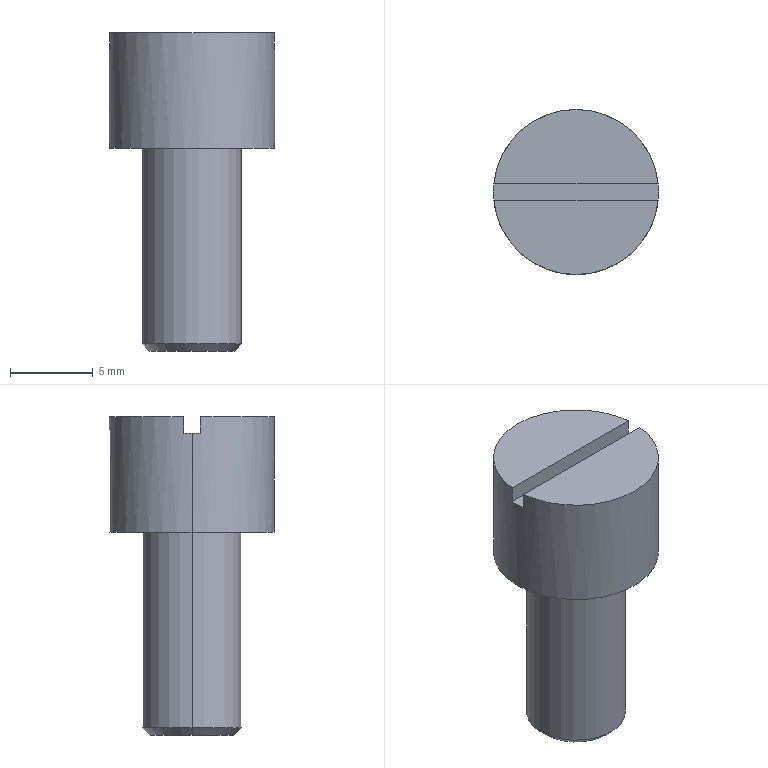Part | Creo | 1 solid | 13 faces | box 10 x 10 x 19.3 mm | volume 885.757 mm3 | plane 7 | cylinder 4 | cone 2 | commonest cylinder face diameters 6 x2 10 x2
STEP:
#1=CARTESIAN_POINT('',(-51.236,1.687,24.177));
#2=VERTEX_POINT('',#1);
#3=CARTESIAN_POINT('',(-41.236,1.687,24.177));
#4=VERTEX_POINT('',#3);
#5=CARTESIAN_POINT('',(-46.236,1.687,24.177));
#6=DIRECTION('',(0.,0.,-1.));
#7=DIRECTION('',(-1.,0.,0.));
#8=AXIS2_PLACEMENT_3D('',#5,#6,#7);
#9=CIRCLE('',#8,5.);
#10=EDGE_CURVE('',#2,#4,#9,.T.);
#11=ORIENTED_EDGE('',*,*,#10,.F.);
#12=CARTESIAN_POINT('',(-46.236,1.687,24.177));
#13=DIRECTION('',(0.,0.,-1.));
#14=DIRECTION('',(1.,0.,0.));
#15=AXIS2_PLACEMENT_3D('',#12,#13,#14);
#16=CIRCLE('',#15,5.);
#17=EDGE_CURVE('',#4,#2,#16,.T.);
#18=ORIENTED_EDGE('',*,*,#17,.F.);
#19=EDGE_LOOP('',(#11,#18));
#20=FACE_OUTER_BOUND('',#19,.F.);
#21=CARTESIAN_POINT('',(-49.236,1.687,24.177));
#22=VERTEX_POINT('',#21);
#23=CARTESIAN_POINT('',(-43.236,1.687,24.177));
#24=VERTEX_POINT('',#23);
#25=CARTESIAN_POINT('',(-46.236,1.687,24.177));
#26=DIRECTION('',(0.,0.,1.));
#27=DIRECTION('',(-1.,0.,0.));
#28=AXIS2_PLACEMENT_3D('',#25,#26,#27);
#29=CIRCLE('',#28,3.);
#30=EDGE_CURVE('',#22,#24,#29,.T.);
#31=ORIENTED_EDGE('',*,*,#30,.F.);
#32=CARTESIAN_POINT('',(-46.236,1.687,24.177));
#33=DIRECTION('',(0.,0.,1.));
#34=DIRECTION('',(1.,0.,0.));
#35=AXIS2_PLACEMENT_3D('',#32,#33,#34);
#36=CIRCLE('',#35,3.);
#37=EDGE_CURVE('',#24,#22,#36,.T.);
#38=ORIENTED_EDGE('',*,*,#37,.F.);
#39=EDGE_LOOP('',(#31,#38));
#40=FACE_BOUND('',#39,.F.);
#41=CARTESIAN_POINT('',(-46.236,1.687,24.177));
#42=DIRECTION('',(0.,0.,-1.));
#43=DIRECTION('',(-1.,0.,0.));
#44=AXIS2_PLACEMENT_3D('',#41,#42,#43);
#45=PLANE('',#44);
#46=ADVANCED_FACE('',(#20,#40),#45,.T.);
#47=CARTESIAN_POINT('',(-41.261,2.187,31.177));
#48=VERTEX_POINT('',#47);
#49=CARTESIAN_POINT('',(-41.261,2.187,30.177));
#50=VERTEX_POINT('',#49);
#51=CARTESIAN_POINT('',(-41.261,2.187,31.177));
#52=DIRECTION('',(0.,0.,-1.));
#53=VECTOR('',#52,1.);
#54=LINE('',#51,#53);
#55=EDGE_CURVE('',#48,#50,#54,.T.);
#56=ORIENTED_EDGE('',*,*,#55,.F.);
#57=CARTESIAN_POINT('',(-51.211,2.187,31.177));
#58=VERTEX_POINT('',#57);
#59=CARTESIAN_POINT('',(-46.236,1.687,31.177));
#60=DIRECTION('',(0.,0.,1.));
#61=DIRECTION('',(0.995,0.1,0.));
#62=AXIS2_PLACEMENT_3D('',#59,#60,#61);
#63=CIRCLE('',#62,5.);
#64=EDGE_CURVE('',#48,#58,#63,.T.);
#65=ORIENTED_EDGE('',*,*,#64,.T.);
#66=CARTESIAN_POINT('',(-51.211,2.187,30.177));
#67=VERTEX_POINT('',#66);
#68=CARTESIAN_POINT('',(-51.211,2.187,30.177));
#69=DIRECTION('',(0.,0.,1.));
#70=VECTOR('',#69,1.);
#71=LINE('',#68,#70);
#72=EDGE_CURVE('',#67,#58,#71,.T.);
#73=ORIENTED_EDGE('',*,*,#72,.F.);
#74=CARTESIAN_POINT('',(-51.236,1.687,30.177));
#75=VERTEX_POINT('',#74);
#76=CARTESIAN_POINT('',(-46.236,1.687,30.177));
#77=DIRECTION('',(0.,0.,1.));
#78=DIRECTION('',(-0.995,0.1,0.));
#79=AXIS2_PLACEMENT_3D('',#76,#77,#78);
#80=CIRCLE('',#79,5.);
#81=EDGE_CURVE('',#67,#75,#80,.T.);
#82=ORIENTED_EDGE('',*,*,#81,.T.);
#83=CARTESIAN_POINT('',(-51.236,1.687,30.177));
#84=DIRECTION('',(-0.000000136,0.,-1.));
#85=VECTOR('',#84,6.);
#86=LINE('',#83,#85);
#87=EDGE_CURVE('',#75,#2,#86,.T.);
#88=ORIENTED_EDGE('',*,*,#87,.T.);
#89=ORIENTED_EDGE('',*,*,#10,.T.);
#90=CARTESIAN_POINT('',(-41.236,1.687,30.177));
#91=VERTEX_POINT('',#90);
#92=CARTESIAN_POINT('',(-41.236,1.687,30.177));
#93=DIRECTION('',(0.,0.,-1.));
#94=VECTOR('',#93,6.);
#95=LINE('',#92,#94);
#96=EDGE_CURVE('',#91,#4,#95,.T.);
#97=ORIENTED_EDGE('',*,*,#96,.F.);
#98=CARTESIAN_POINT('',(-46.236,1.687,30.177));
#99=DIRECTION('',(0.,0.,1.));
#100=DIRECTION('',(1.,0.,0.));
#101=AXIS2_PLACEMENT_3D('',#98,#99,#100);
#102=CIRCLE('',#101,5.);
#103=EDGE_CURVE('',#91,#50,#102,.T.);
#104=ORIENTED_EDGE('',*,*,#103,.T.);
#105=EDGE_LOOP('',(#56,#65,#73,#82,#88,#89,#97,#104));
#106=FACE_OUTER_BOUND('',#105,.F.);
#107=CARTESIAN_POINT('',(-46.236,1.687,28.177));
#108=DIRECTION('',(0.,0.,-1.));
#109=DIRECTION('',(-1.,0.,0.));
#110=AXIS2_PLACEMENT_3D('',#107,#108,#109);
#111=CYLINDRICAL_SURFACE('',#110,5.);
#112=ADVANCED_FACE('',(#106),#111,.T.);
#113=ORIENTED_EDGE('',*,*,#72,.T.);
#114=CARTESIAN_POINT('',(-41.261,2.187,31.177));
#115=DIRECTION('',(-1.,0.,0.));
#116=VECTOR('',#115,9.95);
#117=LINE('',#114,#116);
#118=EDGE_CURVE('',#48,#58,#117,.T.);
#119=ORIENTED_EDGE('',*,*,#118,.F.);
#120=ORIENTED_EDGE('',*,*,#55,.T.);
#121=CARTESIAN_POINT('',(-41.261,2.187,30.177));
#122=DIRECTION('',(-1.,0.,0.));
#123=VECTOR('',#122,9.95);
#124=LINE('',#121,#123);
#125=EDGE_CURVE('',#50,#67,#124,.T.);
#126=ORIENTED_EDGE('',*,*,#125,.T.);
#127=EDGE_LOOP('',(#113,#119,#120,#126));
#128=FACE_OUTER_BOUND('',#127,.F.);
#129=CARTESIAN_POINT('',(-46.236,2.187,31.177));
#130=DIRECTION('',(0.,1.,0.));
#131=DIRECTION('',(0.,0.,1.));
#132=AXIS2_PLACEMENT_3D('',#129,#130,#131);
#133=PLANE('',#132);
#134=ADVANCED_FACE('',(#128),#133,.F.);
#135=ORIENTED_EDGE('',*,*,#64,.F.);
#136=ORIENTED_EDGE('',*,*,#118,.T.);
#137=EDGE_LOOP('',(#135,#136));
#138=FACE_OUTER_BOUND('',#137,.F.);
#139=CARTESIAN_POINT('',(-46.236,1.687,31.177));
#140=DIRECTION('',(0.,0.,-1.));
#141=DIRECTION('',(-1.,0.,0.));
#142=AXIS2_PLACEMENT_3D('',#139,#140,#141);
#143=PLANE('',#142);
#144=ADVANCED_FACE('',(#138),#143,.F.);
#145=CARTESIAN_POINT('',(-51.211,1.187,30.177));
#146=VERTEX_POINT('',#145);
#147=CARTESIAN_POINT('',(-46.236,1.687,30.177));
#148=DIRECTION('',(0.,0.,1.));
#149=DIRECTION('',(-1.,0.,0.));
#150=AXIS2_PLACEMENT_3D('',#147,#148,#149);
#151=CIRCLE('',#150,5.);
#152=EDGE_CURVE('',#75,#146,#151,.T.);
#153=ORIENTED_EDGE('',*,*,#152,.F.);
#154=ORIENTED_EDGE('',*,*,#81,.F.);
#155=ORIENTED_EDGE('',*,*,#125,.F.);
#156=ORIENTED_EDGE('',*,*,#103,.F.);
#157=CARTESIAN_POINT('',(-41.261,1.187,30.177));
#158=VERTEX_POINT('',#157);
#159=CARTESIAN_POINT('',(-46.236,1.687,30.177));
#160=DIRECTION('',(0.,0.,1.));
#161=DIRECTION('',(0.995,-0.1,0.));
#162=AXIS2_PLACEMENT_3D('',#159,#160,#161);
#163=CIRCLE('',#162,5.);
#164=EDGE_CURVE('',#158,#91,#163,.T.);
#165=ORIENTED_EDGE('',*,*,#164,.F.);
#166=CARTESIAN_POINT('',(-41.261,1.187,30.177));
#167=DIRECTION('',(-1.,0.,0.));
#168=VECTOR('',#167,9.95);
#169=LINE('',#166,#168);
#170=EDGE_CURVE('',#158,#146,#169,.T.);
#171=ORIENTED_EDGE('',*,*,#170,.T.);
#172=EDGE_LOOP('',(#153,#154,#155,#156,#165,#171));
#173=FACE_OUTER_BOUND('',#172,.F.);
#174=CARTESIAN_POINT('',(-46.236,1.687,30.177));
#175=DIRECTION('',(0.,0.,-1.));
#176=DIRECTION('',(-1.,0.,0.));
#177=AXIS2_PLACEMENT_3D('',#174,#175,#176);
#178=PLANE('',#177);
#179=ADVANCED_FACE('',(#173),#178,.F.);
#180=ORIENTED_EDGE('',*,*,#164,.T.);
#181=ORIENTED_EDGE('',*,*,#96,.T.);
#182=ORIENTED_EDGE('',*,*,#17,.T.);
#183=ORIENTED_EDGE('',*,*,#87,.F.);
#184=ORIENTED_EDGE('',*,*,#152,.T.);
#185=CARTESIAN_POINT('',(-51.211,1.187,31.177));
#186=VERTEX_POINT('',#185);
#187=CARTESIAN_POINT('',(-51.211,1.187,31.177));
#188=DIRECTION('',(0.,0.,-1.));
#189=VECTOR('',#188,1.);
#190=LINE('',#187,#189);
#191=EDGE_CURVE('',#186,#146,#190,.T.);
#192=ORIENTED_EDGE('',*,*,#191,.F.);
#193=CARTESIAN_POINT('',(-41.261,1.187,31.177));
#194=VERTEX_POINT('',#193);
#195=CARTESIAN_POINT('',(-46.236,1.687,31.177));
#196=DIRECTION('',(0.,0.,1.));
#197=DIRECTION('',(-0.995,-0.1,0.));
#198=AXIS2_PLACEMENT_3D('',#195,#196,#197);
#199=CIRCLE('',#198,5.);
#200=EDGE_CURVE('',#186,#194,#199,.T.);
#201=ORIENTED_EDGE('',*,*,#200,.T.);
#202=CARTESIAN_POINT('',(-41.261,1.187,30.177));
#203=DIRECTION('',(0.,0.,1.));
#204=VECTOR('',#203,1.);
#205=LINE('',#202,#204);
#206=EDGE_CURVE('',#158,#194,#205,.T.);
#207=ORIENTED_EDGE('',*,*,#206,.F.);
#208=EDGE_LOOP('',(#180,#181,#182,#183,#184,#192,#201,#207));
#209=FACE_OUTER_BOUND('',#208,.F.);
#210=CARTESIAN_POINT('',(-46.236,1.687,28.177));
#211=DIRECTION('',(0.,0.,-1.));
#212=DIRECTION('',(-1.,0.,0.));
#213=AXIS2_PLACEMENT_3D('',#210,#211,#212);
#214=CYLINDRICAL_SURFACE('',#213,5.);
#215=ADVANCED_FACE('',(#209),#214,.T.);
#216=ORIENTED_EDGE('',*,*,#170,.F.);
#217=ORIENTED_EDGE('',*,*,#206,.T.);
#218=CARTESIAN_POINT('',(-41.261,1.187,31.177));
#219=DIRECTION('',(-1.,0.,0.));
#220=VECTOR('',#219,9.95);
#221=LINE('',#218,#220);
#222=EDGE_CURVE('',#194,#186,#221,.T.);
#223=ORIENTED_EDGE('',*,*,#222,.T.);
#224=ORIENTED_EDGE('',*,*,#191,.T.);
#225=EDGE_LOOP('',(#216,#217,#223,#224));
#226=FACE_OUTER_BOUND('',#225,.F.);
#227=CARTESIAN_POINT('',(-46.236,1.187,31.177));
#228=DIRECTION('',(0.,1.,0.));
#229=DIRECTION('',(0.,0.,1.));
#230=AXIS2_PLACEMENT_3D('',#227,#228,#229);
#231=PLANE('',#230);
#232=ADVANCED_FACE('',(#226),#231,.T.);
#233=ORIENTED_EDGE('',*,*,#222,.F.);
#234=ORIENTED_EDGE('',*,*,#200,.F.);
#235=EDGE_LOOP('',(#233,#234));
#236=FACE_OUTER_BOUND('',#235,.F.);
#237=CARTESIAN_POINT('',(-46.236,1.687,31.177));
#238=DIRECTION('',(0.,0.,-1.));
#239=DIRECTION('',(-1.,0.,0.));
#240=AXIS2_PLACEMENT_3D('',#237,#238,#239);
#241=PLANE('',#240);
#242=ADVANCED_FACE('',(#236),#241,.F.);
#243=ORIENTED_EDGE('',*,*,#30,.T.);
#244=CARTESIAN_POINT('',(-43.236,1.687,12.327));
#245=VERTEX_POINT('',#244);
#246=CARTESIAN_POINT('',(-43.236,1.687,24.177));
#247=DIRECTION('',(0.,0.,-1.));
#248=VECTOR('',#247,11.85);
#249=LINE('',#246,#248);
#250=EDGE_CURVE('',#24,#245,#249,.T.);
#251=ORIENTED_EDGE('',*,*,#250,.T.);
#252=CARTESIAN_POINT('',(-49.236,1.687,12.327));
#253=VERTEX_POINT('',#252);
#254=CARTESIAN_POINT('',(-46.236,1.687,12.327));
#255=DIRECTION('',(0.,0.,-1.));
#256=DIRECTION('',(1.,0.,0.));
#257=AXIS2_PLACEMENT_3D('',#254,#255,#256);
#258=CIRCLE('',#257,3.);
#259=EDGE_CURVE('',#245,#253,#258,.T.);
#260=ORIENTED_EDGE('',*,*,#259,.T.);
#261=CARTESIAN_POINT('',(-49.236,1.687,24.177));
#262=DIRECTION('',(0.,0.,-1.));
#263=VECTOR('',#262,11.85);
#264=LINE('',#261,#263);
#265=EDGE_CURVE('',#22,#253,#264,.T.);
#266=ORIENTED_EDGE('',*,*,#265,.F.);
#267=EDGE_LOOP('',(#243,#251,#260,#266));
#268=FACE_OUTER_BOUND('',#267,.F.);
#269=CARTESIAN_POINT('',(-46.236,1.687,31.177));
#270=DIRECTION('',(0.,0.,-1.));
#271=DIRECTION('',(-1.,0.,0.));
#272=AXIS2_PLACEMENT_3D('',#269,#270,#271);
#273=CYLINDRICAL_SURFACE('',#272,3.);
#274=ADVANCED_FACE('',(#268),#273,.T.);
#275=ORIENTED_EDGE('',*,*,#37,.T.);
#276=ORIENTED_EDGE('',*,*,#265,.T.);
#277=CARTESIAN_POINT('',(-46.236,1.687,12.327));
#278=DIRECTION('',(0.,0.,-1.));
#279=DIRECTION('',(-1.,0.,0.));
#280=AXIS2_PLACEMENT_3D('',#277,#278,#279);
#281=CIRCLE('',#280,3.);
#282=EDGE_CURVE('',#253,#245,#281,.T.);
#283=ORIENTED_EDGE('',*,*,#282,.T.);
#284=ORIENTED_EDGE('',*,*,#250,.F.);
#285=EDGE_LOOP('',(#275,#276,#283,#284));
#286=FACE_OUTER_BOUND('',#285,.F.);
#287=CARTESIAN_POINT('',(-46.236,1.687,31.177));
#288=DIRECTION('',(0.,0.,-1.));
#289=DIRECTION('',(-1.,0.,0.));
#290=AXIS2_PLACEMENT_3D('',#287,#288,#289);
#291=CYLINDRICAL_SURFACE('',#290,3.);
#292=ADVANCED_FACE('',(#286),#291,.T.);
#293=CARTESIAN_POINT('',(-48.786,1.687,11.877));
#294=VERTEX_POINT('',#293);
#295=CARTESIAN_POINT('',(-43.686,1.687,11.877));
#296=VERTEX_POINT('',#295);
#297=CARTESIAN_POINT('',(-46.236,1.687,11.877));
#298=DIRECTION('',(0.,0.,-1.));
#299=DIRECTION('',(-1.,0.,0.));
#300=AXIS2_PLACEMENT_3D('',#297,#298,#299);
#301=CIRCLE('',#300,2.55);
#302=EDGE_CURVE('',#294,#296,#301,.T.);
#303=ORIENTED_EDGE('',*,*,#302,.T.);
#304=CARTESIAN_POINT('',(-43.686,1.687,11.877));
#305=DIRECTION('',(0.7071,0.,0.7071));
#306=VECTOR('',#305,0.6364);
#307=LINE('',#304,#306);
#308=EDGE_CURVE('',#296,#245,#307,.T.);
#309=ORIENTED_EDGE('',*,*,#308,.T.);
#310=ORIENTED_EDGE('',*,*,#282,.F.);
#311=CARTESIAN_POINT('',(-48.786,1.687,11.877));
#312=DIRECTION('',(-0.7071,0.,0.7071));
#313=VECTOR('',#312,0.6364);
#314=LINE('',#311,#313);
#315=EDGE_CURVE('',#294,#253,#314,.T.);
#316=ORIENTED_EDGE('',*,*,#315,.F.);
#317=EDGE_LOOP('',(#303,#309,#310,#316));
#318=FACE_OUTER_BOUND('',#317,.F.);
#319=CARTESIAN_POINT('',(-46.236,1.687,12.102));
#320=DIRECTION('',(0.,0.,1.));
#321=DIRECTION('',(1.,0.,0.));
#322=AXIS2_PLACEMENT_3D('',#319,#320,#321);
#323=CONICAL_SURFACE('',#322,2.775,45.);
#324=ADVANCED_FACE('',(#318),#323,.T.);
#325=ORIENTED_EDGE('',*,*,#302,.F.);
#326=CARTESIAN_POINT('',(-46.236,1.687,11.877));
#327=DIRECTION('',(0.,0.,-1.));
#328=DIRECTION('',(1.,0.,0.));
#329=AXIS2_PLACEMENT_3D('',#326,#327,#328);
#330=CIRCLE('',#329,2.55);
#331=EDGE_CURVE('',#296,#294,#330,.T.);
#332=ORIENTED_EDGE('',*,*,#331,.F.);
#333=EDGE_LOOP('',(#325,#332));
#334=FACE_OUTER_BOUND('',#333,.F.);
#335=CARTESIAN_POINT('',(-46.236,1.687,11.877));
#336=DIRECTION('',(0.,0.,-1.));
#337=DIRECTION('',(-1.,0.,0.));
#338=AXIS2_PLACEMENT_3D('',#335,#336,#337);
#339=PLANE('',#338);
#340=ADVANCED_FACE('',(#334),#339,.T.);
#341=ORIENTED_EDGE('',*,*,#331,.T.);
#342=ORIENTED_EDGE('',*,*,#315,.T.);
#343=ORIENTED_EDGE('',*,*,#259,.F.);
#344=ORIENTED_EDGE('',*,*,#308,.F.);
#345=EDGE_LOOP('',(#341,#342,#343,#344));
#346=FACE_OUTER_BOUND('',#345,.F.);
#347=CARTESIAN_POINT('',(-46.236,1.687,12.102));
#348=DIRECTION('',(0.,0.,1.));
#349=DIRECTION('',(1.,0.,0.));
#350=AXIS2_PLACEMENT_3D('',#347,#348,#349);
#351=CONICAL_SURFACE('',#350,2.775,45.);
#352=ADVANCED_FACE('',(#346),#351,.T.);
#353=CLOSED_SHELL('',(#46,#112,#134,#144,#179,#215,#232,#242,#274,#292,#324,#340,#352));
#354=MANIFOLD_SOLID_BREP('',#353);
#355=(LENGTH_UNIT()NAMED_UNIT(*)SI_UNIT(.MILLI.,.METRE.));
#356=UNCERTAINTY_MEASURE_WITH_UNIT(LENGTH_MEASURE(0.002393),#355,'','');
#357=(NAMED_UNIT(*)PLANE_ANGLE_UNIT()SI_UNIT($,.RADIAN.));
#358=PLANE_ANGLE_MEASURE_WITH_UNIT(PLANE_ANGLE_MEASURE(0.01745),#357);
#359=(CONVERSION_BASED_UNIT('DEGREE',#358)NAMED_UNIT(*)PLANE_ANGLE_UNIT());
#360=(NAMED_UNIT(*)SI_UNIT($,.STERADIAN.)SOLID_ANGLE_UNIT());
#361=(GEOMETRIC_REPRESENTATION_CONTEXT(3)GLOBAL_UNCERTAINTY_ASSIGNED_CONTEXT((#356))GLOBAL_UNIT_ASSIGNED_CONTEXT((#355,#359,#360))REPRESENTATION_CONTEXT('',''));
#362=ADVANCED_BREP_SHAPE_REPRESENTATION('',(#354),#361);